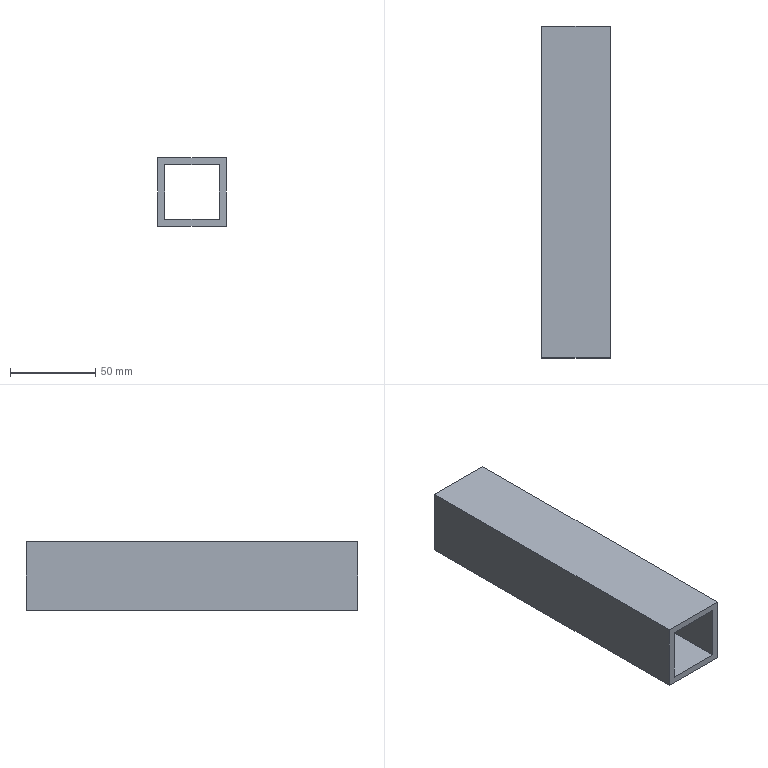Part | NX | features solid 2 | 1 solid | 10 faces | box 40 x 195 x 40 mm | volume 112320 mm3 | plane 10
STEP:
#1=CARTESIAN_POINT('',(-1176.,-370.,-81.));
#2=VERTEX_POINT('',#1);
#3=CARTESIAN_POINT('',(-1176.,-565.,-81.));
#4=VERTEX_POINT('',#3);
#5=CARTESIAN_POINT('',(-1176.,-50.,-81.));
#6=DIRECTION('',(0.,-1.,0.));
#7=VECTOR('',#6,1000.);
#8=LINE('',#5,#7);
#9=EDGE_CURVE('',#2,#4,#8,.T.);
#10=ORIENTED_EDGE('',*,*,#9,.T.);
#11=CARTESIAN_POINT('',(-1144.,-565.,-81.));
#12=VERTEX_POINT('',#11);
#13=CARTESIAN_POINT('',(149.393,-565.,-81.));
#14=DIRECTION('',(1.,0.,0.));
#15=VECTOR('',#14,1000.);
#16=LINE('',#13,#15);
#17=EDGE_CURVE('',#4,#12,#16,.T.);
#18=ORIENTED_EDGE('',*,*,#17,.T.);
#19=CARTESIAN_POINT('',(-1144.,-370.,-81.));
#20=VERTEX_POINT('',#19);
#21=CARTESIAN_POINT('',(-1144.,-50.,-81.));
#22=DIRECTION('',(0.,-1.,0.));
#23=VECTOR('',#22,1000.);
#24=LINE('',#21,#23);
#25=EDGE_CURVE('',#20,#12,#24,.T.);
#26=ORIENTED_EDGE('',*,*,#25,.F.);
#27=CARTESIAN_POINT('',(-180.607,-370.,-81.));
#28=DIRECTION('',(-1.,0.,0.));
#29=VECTOR('',#28,1000.);
#30=LINE('',#27,#29);
#31=EDGE_CURVE('',#2,#20,#30,.F.);
#32=ORIENTED_EDGE('',*,*,#31,.F.);
#33=EDGE_LOOP('',(#10,#18,#26,#32));
#34=FACE_BOUND('',#33,.T.);
#35=CARTESIAN_POINT('',(-1180.,-50.,-81.));
#36=DIRECTION('',(0.,0.,-1.));
#37=DIRECTION('',(-1.,0.,0.));
#38=AXIS2_PLACEMENT_3D('',#35,#36,#37);
#39=PLANE('',#38);
#40=ADVANCED_FACE('',(#34),#39,.F.);
#41=CARTESIAN_POINT('',(-1144.,-370.,-49.));
#42=VERTEX_POINT('',#41);
#43=CARTESIAN_POINT('',(-1144.,-370.,-70.));
#44=DIRECTION('',(0.,0.,1.));
#45=VECTOR('',#44,1000.);
#46=LINE('',#43,#45);
#47=EDGE_CURVE('',#42,#20,#46,.F.);
#48=ORIENTED_EDGE('',*,*,#47,.T.);
#49=ORIENTED_EDGE('',*,*,#25,.T.);
#50=CARTESIAN_POINT('',(-1144.,-565.,-49.));
#51=VERTEX_POINT('',#50);
#52=CARTESIAN_POINT('',(-1144.,-565.,-40.));
#53=DIRECTION('',(0.,0.,-1.));
#54=VECTOR('',#53,1000.);
#55=LINE('',#52,#54);
#56=EDGE_CURVE('',#51,#12,#55,.T.);
#57=ORIENTED_EDGE('',*,*,#56,.F.);
#58=CARTESIAN_POINT('',(-1144.,-50.,-49.));
#59=DIRECTION('',(0.,-1.,0.));
#60=VECTOR('',#59,1000.);
#61=LINE('',#58,#60);
#62=EDGE_CURVE('',#42,#51,#61,.T.);
#63=ORIENTED_EDGE('',*,*,#62,.F.);
#64=EDGE_LOOP('',(#48,#49,#57,#63));
#65=FACE_BOUND('',#64,.T.);
#66=CARTESIAN_POINT('',(-1144.,-50.,-45.));
#67=DIRECTION('',(-1.,0.,0.));
#68=DIRECTION('',(0.,0.,1.));
#69=AXIS2_PLACEMENT_3D('',#66,#67,#68);
#70=PLANE('',#69);
#71=ADVANCED_FACE('',(#65),#70,.T.);
#72=CARTESIAN_POINT('',(-1176.,-370.,-49.));
#73=VERTEX_POINT('',#72);
#74=CARTESIAN_POINT('',(-180.607,-370.,-49.));
#75=DIRECTION('',(-1.,0.,0.));
#76=VECTOR('',#75,1000.);
#77=LINE('',#74,#76);
#78=EDGE_CURVE('',#73,#42,#77,.F.);
#79=ORIENTED_EDGE('',*,*,#78,.T.);
#80=ORIENTED_EDGE('',*,*,#62,.T.);
#81=CARTESIAN_POINT('',(-1176.,-565.,-49.));
#82=VERTEX_POINT('',#81);
#83=CARTESIAN_POINT('',(149.393,-565.,-49.));
#84=DIRECTION('',(1.,0.,0.));
#85=VECTOR('',#84,1000.);
#86=LINE('',#83,#85);
#87=EDGE_CURVE('',#82,#51,#86,.T.);
#88=ORIENTED_EDGE('',*,*,#87,.F.);
#89=CARTESIAN_POINT('',(-1176.,-50.,-49.));
#90=DIRECTION('',(0.,-1.,0.));
#91=VECTOR('',#90,1000.);
#92=LINE('',#89,#91);
#93=EDGE_CURVE('',#73,#82,#92,.T.);
#94=ORIENTED_EDGE('',*,*,#93,.F.);
#95=EDGE_LOOP('',(#79,#80,#88,#94));
#96=FACE_BOUND('',#95,.T.);
#97=CARTESIAN_POINT('',(-1180.,-50.,-49.));
#98=DIRECTION('',(0.,0.,-1.));
#99=DIRECTION('',(-1.,0.,0.));
#100=AXIS2_PLACEMENT_3D('',#97,#98,#99);
#101=PLANE('',#100);
#102=ADVANCED_FACE('',(#96),#101,.T.);
#103=ORIENTED_EDGE('',*,*,#93,.T.);
#104=CARTESIAN_POINT('',(-1176.,-565.,-40.));
#105=DIRECTION('',(0.,0.,-1.));
#106=VECTOR('',#105,1000.);
#107=LINE('',#104,#106);
#108=EDGE_CURVE('',#82,#4,#107,.T.);
#109=ORIENTED_EDGE('',*,*,#108,.T.);
#110=ORIENTED_EDGE('',*,*,#9,.F.);
#111=CARTESIAN_POINT('',(-1176.,-370.,-70.));
#112=DIRECTION('',(0.,0.,1.));
#113=VECTOR('',#112,1000.);
#114=LINE('',#111,#113);
#115=EDGE_CURVE('',#73,#2,#114,.F.);
#116=ORIENTED_EDGE('',*,*,#115,.F.);
#117=EDGE_LOOP('',(#103,#109,#110,#116));
#118=FACE_BOUND('',#117,.T.);
#119=CARTESIAN_POINT('',(-1176.,-50.,-45.));
#120=DIRECTION('',(-1.,0.,0.));
#121=DIRECTION('',(0.,0.,1.));
#122=AXIS2_PLACEMENT_3D('',#119,#120,#121);
#123=PLANE('',#122);
#124=ADVANCED_FACE('',(#118),#123,.F.);
#125=CARTESIAN_POINT('',(-1180.,-370.,-85.));
#126=VERTEX_POINT('',#125);
#127=CARTESIAN_POINT('',(-1180.,-565.,-85.));
#128=VERTEX_POINT('',#127);
#129=CARTESIAN_POINT('',(-1180.,-450.,-85.));
#130=DIRECTION('',(0.,-1.,0.));
#131=VECTOR('',#130,1000.);
#132=LINE('',#129,#131);
#133=EDGE_CURVE('',#126,#128,#132,.T.);
#134=ORIENTED_EDGE('',*,*,#133,.T.);
#135=CARTESIAN_POINT('',(-1180.,-565.,-45.));
#136=VERTEX_POINT('',#135);
#137=CARTESIAN_POINT('',(-1180.,-565.,-40.));
#138=DIRECTION('',(0.,0.,-1.));
#139=VECTOR('',#138,1000.);
#140=LINE('',#137,#139);
#141=EDGE_CURVE('',#136,#128,#140,.T.);
#142=ORIENTED_EDGE('',*,*,#141,.F.);
#143=CARTESIAN_POINT('',(-1180.,-370.,-45.));
#144=VERTEX_POINT('',#143);
#145=CARTESIAN_POINT('',(-1180.,-450.,-45.));
#146=DIRECTION('',(0.,1.,0.));
#147=VECTOR('',#146,1000.);
#148=LINE('',#145,#147);
#149=EDGE_CURVE('',#144,#136,#148,.F.);
#150=ORIENTED_EDGE('',*,*,#149,.F.);
#151=CARTESIAN_POINT('',(-1180.,-370.,-70.));
#152=DIRECTION('',(0.,0.,1.));
#153=VECTOR('',#152,1000.);
#154=LINE('',#151,#153);
#155=EDGE_CURVE('',#144,#126,#154,.F.);
#156=ORIENTED_EDGE('',*,*,#155,.T.);
#157=EDGE_LOOP('',(#134,#142,#150,#156));
#158=FACE_BOUND('',#157,.T.);
#159=CARTESIAN_POINT('',(-1180.,-450.,-40.));
#160=DIRECTION('',(-1.,0.,0.));
#161=DIRECTION('',(0.,0.,-1.));
#162=AXIS2_PLACEMENT_3D('',#159,#160,#161);
#163=PLANE('',#162);
#164=ADVANCED_FACE('',(#158),#163,.T.);
#165=CARTESIAN_POINT('',(-1140.,-370.,-45.));
#166=VERTEX_POINT('',#165);
#167=CARTESIAN_POINT('',(-1185.,-370.,-45.));
#168=DIRECTION('',(1.,0.,0.));
#169=VECTOR('',#168,1000.);
#170=LINE('',#167,#169);
#171=EDGE_CURVE('',#144,#166,#170,.T.);
#172=ORIENTED_EDGE('',*,*,#171,.F.);
#173=ORIENTED_EDGE('',*,*,#149,.T.);
#174=CARTESIAN_POINT('',(-1140.,-565.,-45.));
#175=VERTEX_POINT('',#174);
#176=CARTESIAN_POINT('',(-1185.,-565.,-45.));
#177=DIRECTION('',(-1.,0.,0.));
#178=VECTOR('',#177,1000.);
#179=LINE('',#176,#178);
#180=EDGE_CURVE('',#136,#175,#179,.F.);
#181=ORIENTED_EDGE('',*,*,#180,.T.);
#182=CARTESIAN_POINT('',(-1140.,-450.,-45.));
#183=DIRECTION('',(0.,-1.,0.));
#184=VECTOR('',#183,1000.);
#185=LINE('',#182,#184);
#186=EDGE_CURVE('',#166,#175,#185,.T.);
#187=ORIENTED_EDGE('',*,*,#186,.F.);
#188=EDGE_LOOP('',(#172,#173,#181,#187));
#189=FACE_BOUND('',#188,.T.);
#190=CARTESIAN_POINT('',(-1185.,-450.,-45.));
#191=DIRECTION('',(0.,0.,-1.));
#192=DIRECTION('',(1.,0.,0.));
#193=AXIS2_PLACEMENT_3D('',#190,#191,#192);
#194=PLANE('',#193);
#195=ADVANCED_FACE('',(#189),#194,.F.);
#196=CARTESIAN_POINT('',(-1140.,-370.,-85.));
#197=VERTEX_POINT('',#196);
#198=CARTESIAN_POINT('',(-1140.,-370.,-40.));
#199=DIRECTION('',(0.,0.,-1.));
#200=VECTOR('',#199,1000.);
#201=LINE('',#198,#200);
#202=EDGE_CURVE('',#166,#197,#201,.T.);
#203=ORIENTED_EDGE('',*,*,#202,.T.);
#204=CARTESIAN_POINT('',(-180.607,-370.,-85.));
#205=DIRECTION('',(-1.,0.,0.));
#206=VECTOR('',#205,1000.);
#207=LINE('',#204,#206);
#208=EDGE_CURVE('',#126,#197,#207,.F.);
#209=ORIENTED_EDGE('',*,*,#208,.F.);
#210=ORIENTED_EDGE('',*,*,#155,.F.);
#211=ORIENTED_EDGE('',*,*,#171,.T.);
#212=EDGE_LOOP('',(#203,#209,#210,#211));
#213=FACE_BOUND('',#212,.T.);
#214=ORIENTED_EDGE('',*,*,#78,.F.);
#215=ORIENTED_EDGE('',*,*,#115,.T.);
#216=ORIENTED_EDGE('',*,*,#31,.T.);
#217=ORIENTED_EDGE('',*,*,#47,.F.);
#218=EDGE_LOOP('',(#214,#215,#216,#217));
#219=FACE_BOUND('',#218,.T.);
#220=CARTESIAN_POINT('',(-180.607,-370.,-70.));
#221=DIRECTION('',(0.,1.,0.));
#222=DIRECTION('',(0.,0.,1.));
#223=AXIS2_PLACEMENT_3D('',#220,#221,#222);
#224=PLANE('',#223);
#225=ADVANCED_FACE('',(#213,#219),#224,.T.);
#226=CARTESIAN_POINT('',(-1140.,-565.,-85.));
#227=VERTEX_POINT('',#226);
#228=CARTESIAN_POINT('',(-1140.,-565.,-40.));
#229=DIRECTION('',(0.,0.,1.));
#230=VECTOR('',#229,1000.);
#231=LINE('',#228,#230);
#232=EDGE_CURVE('',#175,#227,#231,.F.);
#233=ORIENTED_EDGE('',*,*,#232,.T.);
#234=CARTESIAN_POINT('',(-1140.,-450.,-85.));
#235=DIRECTION('',(0.,1.,0.));
#236=VECTOR('',#235,1000.);
#237=LINE('',#234,#236);
#238=EDGE_CURVE('',#197,#227,#237,.F.);
#239=ORIENTED_EDGE('',*,*,#238,.F.);
#240=ORIENTED_EDGE('',*,*,#202,.F.);
#241=ORIENTED_EDGE('',*,*,#186,.T.);
#242=EDGE_LOOP('',(#233,#239,#240,#241));
#243=FACE_BOUND('',#242,.T.);
#244=CARTESIAN_POINT('',(-1140.,-450.,-40.));
#245=DIRECTION('',(-1.,0.,0.));
#246=DIRECTION('',(0.,0.,-1.));
#247=AXIS2_PLACEMENT_3D('',#244,#245,#246);
#248=PLANE('',#247);
#249=ADVANCED_FACE('',(#243),#248,.F.);
#250=ORIENTED_EDGE('',*,*,#238,.T.);
#251=CARTESIAN_POINT('',(149.393,-565.,-85.));
#252=DIRECTION('',(1.,0.,0.));
#253=VECTOR('',#252,1000.);
#254=LINE('',#251,#253);
#255=EDGE_CURVE('',#128,#227,#254,.T.);
#256=ORIENTED_EDGE('',*,*,#255,.F.);
#257=ORIENTED_EDGE('',*,*,#133,.F.);
#258=ORIENTED_EDGE('',*,*,#208,.T.);
#259=EDGE_LOOP('',(#250,#256,#257,#258));
#260=FACE_BOUND('',#259,.T.);
#261=CARTESIAN_POINT('',(-1185.,-450.,-85.));
#262=DIRECTION('',(0.,0.,-1.));
#263=DIRECTION('',(1.,0.,0.));
#264=AXIS2_PLACEMENT_3D('',#261,#262,#263);
#265=PLANE('',#264);
#266=ADVANCED_FACE('',(#260),#265,.T.);
#267=ORIENTED_EDGE('',*,*,#255,.T.);
#268=ORIENTED_EDGE('',*,*,#232,.F.);
#269=ORIENTED_EDGE('',*,*,#180,.F.);
#270=ORIENTED_EDGE('',*,*,#141,.T.);
#271=EDGE_LOOP('',(#267,#268,#269,#270));
#272=FACE_BOUND('',#271,.T.);
#273=ORIENTED_EDGE('',*,*,#108,.F.);
#274=ORIENTED_EDGE('',*,*,#87,.T.);
#275=ORIENTED_EDGE('',*,*,#56,.T.);
#276=ORIENTED_EDGE('',*,*,#17,.F.);
#277=EDGE_LOOP('',(#273,#274,#275,#276));
#278=FACE_BOUND('',#277,.T.);
#279=CARTESIAN_POINT('',(149.393,-565.,-40.));
#280=DIRECTION('',(0.,-1.,0.));
#281=DIRECTION('',(0.,0.,-1.));
#282=AXIS2_PLACEMENT_3D('',#279,#280,#281);
#283=PLANE('',#282);
#284=ADVANCED_FACE('',(#272,#278),#283,.T.);
#285=CLOSED_SHELL('',(#40,#71,#102,#124,#164,#195,#225,#249,#266,#284));
#286=MANIFOLD_SOLID_BREP('',#285);
#287=(LENGTH_UNIT()NAMED_UNIT(*)SI_UNIT(.MILLI.,.METRE.));
#288=UNCERTAINTY_MEASURE_WITH_UNIT(LENGTH_MEASURE(0.00001),#287,'','');
#289=(NAMED_UNIT(*)PLANE_ANGLE_UNIT()SI_UNIT($,.RADIAN.));
#290=(NAMED_UNIT(*)SI_UNIT($,.STERADIAN.)SOLID_ANGLE_UNIT());
#291=(GEOMETRIC_REPRESENTATION_CONTEXT(3)GLOBAL_UNCERTAINTY_ASSIGNED_CONTEXT((#288))GLOBAL_UNIT_ASSIGNED_CONTEXT((#287,#289,#290))REPRESENTATION_CONTEXT('',''));
#292=ADVANCED_BREP_SHAPE_REPRESENTATION('',(#286),#291);